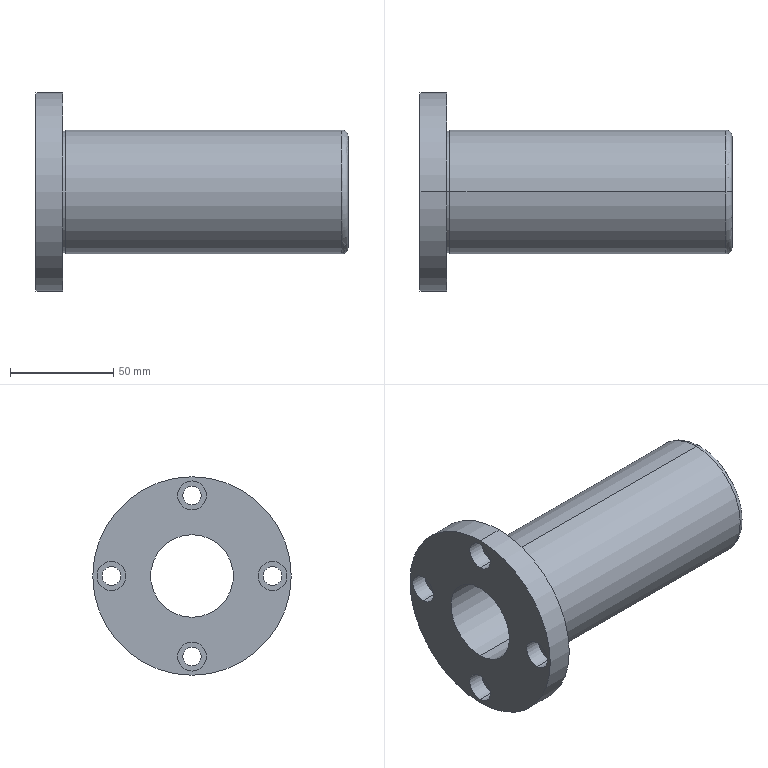Part | SolidWorks | features BaseBody 1 | 1 solid | 34 faces | box 151 x 96 x 96 mm | volume 287800 mm3 | cylinder 24 | plane 8 | torus 2 | commonest cylinder face diameters 9 x8 14 x8 40 x2 59 x2 60 x2 96 x2
STEP:
#1=CARTESIAN_POINT('',(148.,0.,30.));
#2=VERTEX_POINT('',#1);
#3=CARTESIAN_POINT('',(148.,0.,-30.));
#4=VERTEX_POINT('',#3);
#5=CARTESIAN_POINT('',(148.,0.,0.));
#6=DIRECTION('',(-1.,0.,0.));
#7=DIRECTION('',(0.,0.,1.));
#8=AXIS2_PLACEMENT_3D('',#5,#6,#7);
#9=CIRCLE('',#8,30.);
#10=EDGE_CURVE('',#2,#4,#9,.T.);
#11=ORIENTED_EDGE('',*,*,#10,.T.);
#12=CARTESIAN_POINT('',(14.5,0.,-30.));
#13=VERTEX_POINT('',#12);
#14=CARTESIAN_POINT('',(151.,0.,-30.));
#15=DIRECTION('',(-1.,0.,0.));
#16=VECTOR('',#15,1000.);
#17=LINE('',#14,#16);
#18=EDGE_CURVE('',#4,#13,#17,.T.);
#19=ORIENTED_EDGE('',*,*,#18,.T.);
#20=CARTESIAN_POINT('',(14.5,0.,30.));
#21=VERTEX_POINT('',#20);
#22=CARTESIAN_POINT('',(14.5,0.,0.));
#23=DIRECTION('',(1.,0.,0.));
#24=DIRECTION('',(0.,0.,1.));
#25=AXIS2_PLACEMENT_3D('',#22,#23,#24);
#26=CIRCLE('',#25,30.);
#27=EDGE_CURVE('',#13,#21,#26,.T.);
#28=ORIENTED_EDGE('',*,*,#27,.T.);
#29=CARTESIAN_POINT('',(151.,0.,30.));
#30=DIRECTION('',(-1.,0.,0.));
#31=VECTOR('',#30,1000.);
#32=LINE('',#29,#31);
#33=EDGE_CURVE('',#2,#21,#32,.T.);
#34=ORIENTED_EDGE('',*,*,#33,.F.);
#35=EDGE_LOOP('',(#11,#19,#28,#34));
#36=FACE_OUTER_BOUND('',#35,.T.);
#37=CARTESIAN_POINT('',(151.,0.,0.));
#38=DIRECTION('',(-1.,0.,0.));
#39=DIRECTION('',(0.,0.,1.));
#40=AXIS2_PLACEMENT_3D('',#37,#38,#39);
#41=CYLINDRICAL_SURFACE('',#40,30.);
#42=ADVANCED_FACE('',(#36),#41,.T.);
#43=ORIENTED_EDGE('',*,*,#10,.F.);
#44=CARTESIAN_POINT('',(151.,0.,27.));
#45=VERTEX_POINT('',#44);
#46=CARTESIAN_POINT('',(148.,0.,27.));
#47=DIRECTION('',(0.,1.,0.));
#48=DIRECTION('',(0.,0.,1.));
#49=AXIS2_PLACEMENT_3D('',#46,#47,#48);
#50=CIRCLE('',#49,3.);
#51=EDGE_CURVE('',#2,#45,#50,.T.);
#52=ORIENTED_EDGE('',*,*,#51,.T.);
#53=CARTESIAN_POINT('',(151.,0.,-27.));
#54=VERTEX_POINT('',#53);
#55=CARTESIAN_POINT('',(151.,0.,0.));
#56=DIRECTION('',(-1.,0.,0.));
#57=DIRECTION('',(0.,0.,-1.));
#58=AXIS2_PLACEMENT_3D('',#55,#56,#57);
#59=CIRCLE('',#58,27.);
#60=EDGE_CURVE('',#45,#54,#59,.T.);
#61=ORIENTED_EDGE('',*,*,#60,.T.);
#62=CARTESIAN_POINT('',(148.,0.,-27.));
#63=DIRECTION('',(0.,-1.,0.));
#64=DIRECTION('',(0.,0.,-1.));
#65=AXIS2_PLACEMENT_3D('',#62,#63,#64);
#66=CIRCLE('',#65,3.);
#67=EDGE_CURVE('',#4,#54,#66,.T.);
#68=ORIENTED_EDGE('',*,*,#67,.F.);
#69=EDGE_LOOP('',(#43,#52,#61,#68));
#70=FACE_OUTER_BOUND('',#69,.T.);
#71=CARTESIAN_POINT('',(148.,0.,0.));
#72=DIRECTION('',(1.,0.,0.));
#73=DIRECTION('',(0.,0.,-1.));
#74=AXIS2_PLACEMENT_3D('',#71,#72,#73);
#75=TOROIDAL_SURFACE('',#74,27.,3.);
#76=ADVANCED_FACE('',(#70),#75,.T.);
#77=CARTESIAN_POINT('',(14.5,0.,-29.5));
#78=VERTEX_POINT('',#77);
#79=CARTESIAN_POINT('',(14.5,0.,29.5));
#80=VERTEX_POINT('',#79);
#81=CARTESIAN_POINT('',(14.5,0.,0.));
#82=DIRECTION('',(1.,0.,0.));
#83=DIRECTION('',(0.,0.,1.));
#84=AXIS2_PLACEMENT_3D('',#81,#82,#83);
#85=CIRCLE('',#84,29.5);
#86=EDGE_CURVE('',#78,#80,#85,.T.);
#87=ORIENTED_EDGE('',*,*,#86,.F.);
#88=CARTESIAN_POINT('',(13.,0.,-29.5));
#89=VERTEX_POINT('',#88);
#90=CARTESIAN_POINT('',(151.,0.,-29.5));
#91=DIRECTION('',(-1.,0.,0.));
#92=VECTOR('',#91,1000.);
#93=LINE('',#90,#92);
#94=EDGE_CURVE('',#78,#89,#93,.T.);
#95=ORIENTED_EDGE('',*,*,#94,.T.);
#96=CARTESIAN_POINT('',(13.,0.,29.5));
#97=VERTEX_POINT('',#96);
#98=CARTESIAN_POINT('',(13.,0.,0.));
#99=DIRECTION('',(1.,0.,0.));
#100=DIRECTION('',(0.,0.,1.));
#101=AXIS2_PLACEMENT_3D('',#98,#99,#100);
#102=CIRCLE('',#101,29.5);
#103=EDGE_CURVE('',#89,#97,#102,.T.);
#104=ORIENTED_EDGE('',*,*,#103,.T.);
#105=CARTESIAN_POINT('',(151.,0.,29.5));
#106=DIRECTION('',(-1.,0.,0.));
#107=VECTOR('',#106,1000.);
#108=LINE('',#105,#107);
#109=EDGE_CURVE('',#80,#97,#108,.T.);
#110=ORIENTED_EDGE('',*,*,#109,.F.);
#111=EDGE_LOOP('',(#87,#95,#104,#110));
#112=FACE_OUTER_BOUND('',#111,.T.);
#113=CARTESIAN_POINT('',(151.,0.,0.));
#114=DIRECTION('',(-1.,0.,0.));
#115=DIRECTION('',(0.,0.,1.));
#116=AXIS2_PLACEMENT_3D('',#113,#114,#115);
#117=CYLINDRICAL_SURFACE('',#116,29.5);
#118=ADVANCED_FACE('',(#112),#117,.T.);
#119=CARTESIAN_POINT('',(151.,0.,-20.));
#120=VERTEX_POINT('',#119);
#121=CARTESIAN_POINT('',(151.,0.,20.));
#122=VERTEX_POINT('',#121);
#123=CARTESIAN_POINT('',(151.,0.,0.));
#124=DIRECTION('',(-1.,0.,0.));
#125=DIRECTION('',(0.,0.,1.));
#126=AXIS2_PLACEMENT_3D('',#123,#124,#125);
#127=CIRCLE('',#126,20.);
#128=EDGE_CURVE('',#120,#122,#127,.T.);
#129=ORIENTED_EDGE('',*,*,#128,.F.);
#130=CARTESIAN_POINT('',(0.,0.,-20.));
#131=VERTEX_POINT('',#130);
#132=CARTESIAN_POINT('',(151.,0.,-20.));
#133=DIRECTION('',(-1.,0.,0.));
#134=VECTOR('',#133,1000.);
#135=LINE('',#132,#134);
#136=EDGE_CURVE('',#120,#131,#135,.T.);
#137=ORIENTED_EDGE('',*,*,#136,.T.);
#138=CARTESIAN_POINT('',(0.,0.,20.));
#139=VERTEX_POINT('',#138);
#140=CARTESIAN_POINT('',(0.,0.,0.));
#141=DIRECTION('',(1.,0.,0.));
#142=DIRECTION('',(0.,0.,1.));
#143=AXIS2_PLACEMENT_3D('',#140,#141,#142);
#144=CIRCLE('',#143,20.);
#145=EDGE_CURVE('',#139,#131,#144,.T.);
#146=ORIENTED_EDGE('',*,*,#145,.F.);
#147=CARTESIAN_POINT('',(151.,0.,20.));
#148=DIRECTION('',(-1.,0.,0.));
#149=VECTOR('',#148,1000.);
#150=LINE('',#147,#149);
#151=EDGE_CURVE('',#122,#139,#150,.T.);
#152=ORIENTED_EDGE('',*,*,#151,.F.);
#153=EDGE_LOOP('',(#129,#137,#146,#152));
#154=FACE_OUTER_BOUND('',#153,.T.);
#155=CARTESIAN_POINT('',(151.,0.,0.));
#156=DIRECTION('',(-1.,0.,0.));
#157=DIRECTION('',(0.,0.,1.));
#158=AXIS2_PLACEMENT_3D('',#155,#156,#157);
#159=CYLINDRICAL_SURFACE('',#158,20.);
#160=ADVANCED_FACE('',(#154),#159,.F.);
#161=CARTESIAN_POINT('',(13.,0.,-48.));
#162=VERTEX_POINT('',#161);
#163=CARTESIAN_POINT('',(13.,0.,48.));
#164=VERTEX_POINT('',#163);
#165=CARTESIAN_POINT('',(13.,0.,0.));
#166=DIRECTION('',(1.,0.,0.));
#167=DIRECTION('',(0.,0.,1.));
#168=AXIS2_PLACEMENT_3D('',#165,#166,#167);
#169=CIRCLE('',#168,48.);
#170=EDGE_CURVE('',#162,#164,#169,.T.);
#171=ORIENTED_EDGE('',*,*,#170,.F.);
#172=CARTESIAN_POINT('',(0.,0.,-48.));
#173=VERTEX_POINT('',#172);
#174=CARTESIAN_POINT('',(151.,0.,-48.));
#175=DIRECTION('',(-1.,0.,0.));
#176=VECTOR('',#175,1000.);
#177=LINE('',#174,#176);
#178=EDGE_CURVE('',#162,#173,#177,.T.);
#179=ORIENTED_EDGE('',*,*,#178,.T.);
#180=CARTESIAN_POINT('',(0.,0.,48.));
#181=VERTEX_POINT('',#180);
#182=CARTESIAN_POINT('',(0.,0.,0.));
#183=DIRECTION('',(1.,0.,0.));
#184=DIRECTION('',(0.,0.,1.));
#185=AXIS2_PLACEMENT_3D('',#182,#183,#184);
#186=CIRCLE('',#185,48.);
#187=EDGE_CURVE('',#173,#181,#186,.T.);
#188=ORIENTED_EDGE('',*,*,#187,.T.);
#189=CARTESIAN_POINT('',(151.,0.,48.));
#190=DIRECTION('',(-1.,0.,0.));
#191=VECTOR('',#190,1000.);
#192=LINE('',#189,#191);
#193=EDGE_CURVE('',#164,#181,#192,.T.);
#194=ORIENTED_EDGE('',*,*,#193,.F.);
#195=EDGE_LOOP('',(#171,#179,#188,#194));
#196=FACE_OUTER_BOUND('',#195,.T.);
#197=CARTESIAN_POINT('',(151.,0.,0.));
#198=DIRECTION('',(-1.,0.,0.));
#199=DIRECTION('',(0.,0.,1.));
#200=AXIS2_PLACEMENT_3D('',#197,#198,#199);
#201=CYLINDRICAL_SURFACE('',#200,48.);
#202=ADVANCED_FACE('',(#196),#201,.T.);
#203=CARTESIAN_POINT('',(13.,39.,-4.5));
#204=VERTEX_POINT('',#203);
#205=CARTESIAN_POINT('',(13.,39.,4.5));
#206=VERTEX_POINT('',#205);
#207=CARTESIAN_POINT('',(13.,39.,0.));
#208=DIRECTION('',(-1.,0.,0.));
#209=DIRECTION('',(0.,0.,1.));
#210=AXIS2_PLACEMENT_3D('',#207,#208,#209);
#211=CIRCLE('',#210,4.5);
#212=EDGE_CURVE('',#204,#206,#211,.T.);
#213=ORIENTED_EDGE('',*,*,#212,.F.);
#214=CARTESIAN_POINT('',(8.1,39.,-4.5));
#215=VERTEX_POINT('',#214);
#216=CARTESIAN_POINT('',(13.,39.,-4.5));
#217=DIRECTION('',(-1.,0.,0.));
#218=VECTOR('',#217,1000.);
#219=LINE('',#216,#218);
#220=EDGE_CURVE('',#204,#215,#219,.T.);
#221=ORIENTED_EDGE('',*,*,#220,.T.);
#222=CARTESIAN_POINT('',(8.1,39.,4.5));
#223=VERTEX_POINT('',#222);
#224=CARTESIAN_POINT('',(8.1,39.,0.));
#225=DIRECTION('',(1.,0.,0.));
#226=DIRECTION('',(0.,0.,1.));
#227=AXIS2_PLACEMENT_3D('',#224,#225,#226);
#228=CIRCLE('',#227,4.5);
#229=EDGE_CURVE('',#223,#215,#228,.T.);
#230=ORIENTED_EDGE('',*,*,#229,.F.);
#231=CARTESIAN_POINT('',(13.,39.,4.5));
#232=DIRECTION('',(-1.,0.,0.));
#233=VECTOR('',#232,1000.);
#234=LINE('',#231,#233);
#235=EDGE_CURVE('',#206,#223,#234,.T.);
#236=ORIENTED_EDGE('',*,*,#235,.F.);
#237=EDGE_LOOP('',(#213,#221,#230,#236));
#238=FACE_OUTER_BOUND('',#237,.T.);
#239=CARTESIAN_POINT('',(13.,39.,0.));
#240=DIRECTION('',(-1.,0.,0.));
#241=DIRECTION('',(0.,0.,1.));
#242=AXIS2_PLACEMENT_3D('',#239,#240,#241);
#243=CYLINDRICAL_SURFACE('',#242,4.5);
#244=ADVANCED_FACE('',(#238),#243,.F.);
#245=CARTESIAN_POINT('',(13.,0.,-43.5));
#246=VERTEX_POINT('',#245);
#247=CARTESIAN_POINT('',(13.,0.,-34.5));
#248=VERTEX_POINT('',#247);
#249=CARTESIAN_POINT('',(13.,0.,-39.));
#250=DIRECTION('',(-1.,0.,0.));
#251=DIRECTION('',(0.,0.,1.));
#252=AXIS2_PLACEMENT_3D('',#249,#250,#251);
#253=CIRCLE('',#252,4.5);
#254=EDGE_CURVE('',#246,#248,#253,.T.);
#255=ORIENTED_EDGE('',*,*,#254,.F.);
#256=CARTESIAN_POINT('',(8.1,0.,-43.5));
#257=VERTEX_POINT('',#256);
#258=CARTESIAN_POINT('',(13.,0.,-43.5));
#259=DIRECTION('',(-1.,0.,0.));
#260=VECTOR('',#259,1000.);
#261=LINE('',#258,#260);
#262=EDGE_CURVE('',#246,#257,#261,.T.);
#263=ORIENTED_EDGE('',*,*,#262,.T.);
#264=CARTESIAN_POINT('',(8.1,0.,-34.5));
#265=VERTEX_POINT('',#264);
#266=CARTESIAN_POINT('',(8.1,0.,-39.));
#267=DIRECTION('',(1.,0.,0.));
#268=DIRECTION('',(0.,0.,1.));
#269=AXIS2_PLACEMENT_3D('',#266,#267,#268);
#270=CIRCLE('',#269,4.5);
#271=EDGE_CURVE('',#265,#257,#270,.T.);
#272=ORIENTED_EDGE('',*,*,#271,.F.);
#273=CARTESIAN_POINT('',(13.,0.,-34.5));
#274=DIRECTION('',(-1.,0.,0.));
#275=VECTOR('',#274,1000.);
#276=LINE('',#273,#275);
#277=EDGE_CURVE('',#248,#265,#276,.T.);
#278=ORIENTED_EDGE('',*,*,#277,.F.);
#279=EDGE_LOOP('',(#255,#263,#272,#278));
#280=FACE_OUTER_BOUND('',#279,.T.);
#281=CARTESIAN_POINT('',(13.,0.,-39.));
#282=DIRECTION('',(-1.,0.,0.));
#283=DIRECTION('',(0.,0.,1.));
#284=AXIS2_PLACEMENT_3D('',#281,#282,#283);
#285=CYLINDRICAL_SURFACE('',#284,4.5);
#286=ADVANCED_FACE('',(#280),#285,.F.);
#287=CARTESIAN_POINT('',(13.,-39.,-4.5));
#288=VERTEX_POINT('',#287);
#289=CARTESIAN_POINT('',(13.,-39.,4.5));
#290=VERTEX_POINT('',#289);
#291=CARTESIAN_POINT('',(13.,-39.,0.));
#292=DIRECTION('',(-1.,0.,0.));
#293=DIRECTION('',(0.,0.,1.));
#294=AXIS2_PLACEMENT_3D('',#291,#292,#293);
#295=CIRCLE('',#294,4.5);
#296=EDGE_CURVE('',#288,#290,#295,.T.);
#297=ORIENTED_EDGE('',*,*,#296,.F.);
#298=CARTESIAN_POINT('',(8.1,-39.,-4.5));
#299=VERTEX_POINT('',#298);
#300=CARTESIAN_POINT('',(13.,-39.,-4.5));
#301=DIRECTION('',(-1.,0.,0.));
#302=VECTOR('',#301,1000.);
#303=LINE('',#300,#302);
#304=EDGE_CURVE('',#288,#299,#303,.T.);
#305=ORIENTED_EDGE('',*,*,#304,.T.);
#306=CARTESIAN_POINT('',(8.1,-39.,4.5));
#307=VERTEX_POINT('',#306);
#308=CARTESIAN_POINT('',(8.1,-39.,0.));
#309=DIRECTION('',(1.,0.,0.));
#310=DIRECTION('',(0.,0.,1.));
#311=AXIS2_PLACEMENT_3D('',#308,#309,#310);
#312=CIRCLE('',#311,4.5);
#313=EDGE_CURVE('',#307,#299,#312,.T.);
#314=ORIENTED_EDGE('',*,*,#313,.F.);
#315=CARTESIAN_POINT('',(13.,-39.,4.5));
#316=DIRECTION('',(-1.,0.,0.));
#317=VECTOR('',#316,1000.);
#318=LINE('',#315,#317);
#319=EDGE_CURVE('',#290,#307,#318,.T.);
#320=ORIENTED_EDGE('',*,*,#319,.F.);
#321=EDGE_LOOP('',(#297,#305,#314,#320));
#322=FACE_OUTER_BOUND('',#321,.T.);
#323=CARTESIAN_POINT('',(13.,-39.,0.));
#324=DIRECTION('',(-1.,0.,0.));
#325=DIRECTION('',(0.,0.,1.));
#326=AXIS2_PLACEMENT_3D('',#323,#324,#325);
#327=CYLINDRICAL_SURFACE('',#326,4.5);
#328=ADVANCED_FACE('',(#322),#327,.F.);
#329=CARTESIAN_POINT('',(13.,0.,34.5));
#330=VERTEX_POINT('',#329);
#331=CARTESIAN_POINT('',(13.,0.,43.5));
#332=VERTEX_POINT('',#331);
#333=CARTESIAN_POINT('',(13.,0.,39.));
#334=DIRECTION('',(-1.,0.,0.));
#335=DIRECTION('',(0.,0.,1.));
#336=AXIS2_PLACEMENT_3D('',#333,#334,#335);
#337=CIRCLE('',#336,4.5);
#338=EDGE_CURVE('',#330,#332,#337,.T.);
#339=ORIENTED_EDGE('',*,*,#338,.F.);
#340=CARTESIAN_POINT('',(8.1,0.,34.5));
#341=VERTEX_POINT('',#340);
#342=CARTESIAN_POINT('',(13.,0.,34.5));
#343=DIRECTION('',(-1.,0.,0.));
#344=VECTOR('',#343,1000.);
#345=LINE('',#342,#344);
#346=EDGE_CURVE('',#330,#341,#345,.T.);
#347=ORIENTED_EDGE('',*,*,#346,.T.);
#348=CARTESIAN_POINT('',(8.1,0.,43.5));
#349=VERTEX_POINT('',#348);
#350=CARTESIAN_POINT('',(8.1,0.,39.));
#351=DIRECTION('',(1.,0.,0.));
#352=DIRECTION('',(0.,0.,1.));
#353=AXIS2_PLACEMENT_3D('',#350,#351,#352);
#354=CIRCLE('',#353,4.5);
#355=EDGE_CURVE('',#349,#341,#354,.T.);
#356=ORIENTED_EDGE('',*,*,#355,.F.);
#357=CARTESIAN_POINT('',(13.,0.,43.5));
#358=DIRECTION('',(-1.,0.,0.));
#359=VECTOR('',#358,1000.);
#360=LINE('',#357,#359);
#361=EDGE_CURVE('',#332,#349,#360,.T.);
#362=ORIENTED_EDGE('',*,*,#361,.F.);
#363=EDGE_LOOP('',(#339,#347,#356,#362));
#364=FACE_OUTER_BOUND('',#363,.T.);
#365=CARTESIAN_POINT('',(13.,0.,39.));
#366=DIRECTION('',(-1.,0.,0.));
#367=DIRECTION('',(0.,0.,1.));
#368=AXIS2_PLACEMENT_3D('',#365,#366,#367);
#369=CYLINDRICAL_SURFACE('',#368,4.5);
#370=ADVANCED_FACE('',(#364),#369,.F.);
#371=CARTESIAN_POINT('',(8.1,39.,-7.));
#372=VERTEX_POINT('',#371);
#373=CARTESIAN_POINT('',(8.1,39.,7.));
#374=VERTEX_POINT('',#373);
#375=CARTESIAN_POINT('',(8.1,39.,0.));
#376=DIRECTION('',(-1.,0.,0.));
#377=DIRECTION('',(0.,0.,1.));
#378=AXIS2_PLACEMENT_3D('',#375,#376,#377);
#379=CIRCLE('',#378,7.);
#380=EDGE_CURVE('',#372,#374,#379,.T.);
#381=ORIENTED_EDGE('',*,*,#380,.F.);
#382=CARTESIAN_POINT('',(0.,39.,-7.));
#383=VERTEX_POINT('',#382);
#384=CARTESIAN_POINT('',(13.,39.,-7.));
#385=DIRECTION('',(-1.,0.,0.));
#386=VECTOR('',#385,1000.);
#387=LINE('',#384,#386);
#388=EDGE_CURVE('',#372,#383,#387,.T.);
#389=ORIENTED_EDGE('',*,*,#388,.T.);
#390=CARTESIAN_POINT('',(0.,39.,7.));
#391=VERTEX_POINT('',#390);
#392=CARTESIAN_POINT('',(0.,39.,0.));
#393=DIRECTION('',(1.,0.,0.));
#394=DIRECTION('',(0.,0.,1.));
#395=AXIS2_PLACEMENT_3D('',#392,#393,#394);
#396=CIRCLE('',#395,7.);
#397=EDGE_CURVE('',#391,#383,#396,.T.);
#398=ORIENTED_EDGE('',*,*,#397,.F.);
#399=CARTESIAN_POINT('',(13.,39.,7.));
#400=DIRECTION('',(-1.,0.,0.));
#401=VECTOR('',#400,1000.);
#402=LINE('',#399,#401);
#403=EDGE_CURVE('',#374,#391,#402,.T.);
#404=ORIENTED_EDGE('',*,*,#403,.F.);
#405=EDGE_LOOP('',(#381,#389,#398,#404));
#406=FACE_OUTER_BOUND('',#405,.T.);
#407=CARTESIAN_POINT('',(13.,39.,0.));
#408=DIRECTION('',(-1.,0.,0.));
#409=DIRECTION('',(0.,0.,1.));
#410=AXIS2_PLACEMENT_3D('',#407,#408,#409);
#411=CYLINDRICAL_SURFACE('',#410,7.);
#412=ADVANCED_FACE('',(#406),#411,.F.);
#413=CARTESIAN_POINT('',(8.1,0.,-46.));
#414=VERTEX_POINT('',#413);
#415=CARTESIAN_POINT('',(8.1,0.,-32.));
#416=VERTEX_POINT('',#415);
#417=CARTESIAN_POINT('',(8.1,0.,-39.));
#418=DIRECTION('',(-1.,0.,0.));
#419=DIRECTION('',(0.,0.,1.));
#420=AXIS2_PLACEMENT_3D('',#417,#418,#419);
#421=CIRCLE('',#420,7.);
#422=EDGE_CURVE('',#414,#416,#421,.T.);
#423=ORIENTED_EDGE('',*,*,#422,.F.);
#424=CARTESIAN_POINT('',(0.,0.,-46.));
#425=VERTEX_POINT('',#424);
#426=CARTESIAN_POINT('',(13.,0.,-46.));
#427=DIRECTION('',(-1.,0.,0.));
#428=VECTOR('',#427,1000.);
#429=LINE('',#426,#428);
#430=EDGE_CURVE('',#414,#425,#429,.T.);
#431=ORIENTED_EDGE('',*,*,#430,.T.);
#432=CARTESIAN_POINT('',(0.,0.,-32.));
#433=VERTEX_POINT('',#432);
#434=CARTESIAN_POINT('',(0.,0.,-39.));
#435=DIRECTION('',(1.,0.,0.));
#436=DIRECTION('',(0.,0.,1.));
#437=AXIS2_PLACEMENT_3D('',#434,#435,#436);
#438=CIRCLE('',#437,7.);
#439=EDGE_CURVE('',#433,#425,#438,.T.);
#440=ORIENTED_EDGE('',*,*,#439,.F.);
#441=CARTESIAN_POINT('',(13.,0.,-32.));
#442=DIRECTION('',(-1.,0.,0.));
#443=VECTOR('',#442,1000.);
#444=LINE('',#441,#443);
#445=EDGE_CURVE('',#416,#433,#444,.T.);
#446=ORIENTED_EDGE('',*,*,#445,.F.);
#447=EDGE_LOOP('',(#423,#431,#440,#446));
#448=FACE_OUTER_BOUND('',#447,.T.);
#449=CARTESIAN_POINT('',(13.,0.,-39.));
#450=DIRECTION('',(-1.,0.,0.));
#451=DIRECTION('',(0.,0.,1.));
#452=AXIS2_PLACEMENT_3D('',#449,#450,#451);
#453=CYLINDRICAL_SURFACE('',#452,7.);
#454=ADVANCED_FACE('',(#448),#453,.F.);
#455=CARTESIAN_POINT('',(8.1,-39.,-7.));
#456=VERTEX_POINT('',#455);
#457=CARTESIAN_POINT('',(8.1,-39.,7.));
#458=VERTEX_POINT('',#457);
#459=CARTESIAN_POINT('',(8.1,-39.,0.));
#460=DIRECTION('',(-1.,0.,0.));
#461=DIRECTION('',(0.,0.,1.));
#462=AXIS2_PLACEMENT_3D('',#459,#460,#461);
#463=CIRCLE('',#462,7.);
#464=EDGE_CURVE('',#456,#458,#463,.T.);
#465=ORIENTED_EDGE('',*,*,#464,.F.);
#466=CARTESIAN_POINT('',(0.,-39.,-7.));
#467=VERTEX_POINT('',#466);
#468=CARTESIAN_POINT('',(13.,-39.,-7.));
#469=DIRECTION('',(-1.,0.,0.));
#470=VECTOR('',#469,1000.);
#471=LINE('',#468,#470);
#472=EDGE_CURVE('',#456,#467,#471,.T.);
#473=ORIENTED_EDGE('',*,*,#472,.T.);
#474=CARTESIAN_POINT('',(0.,-39.,7.));
#475=VERTEX_POINT('',#474);
#476=CARTESIAN_POINT('',(0.,-39.,0.));
#477=DIRECTION('',(1.,0.,0.));
#478=DIRECTION('',(0.,0.,1.));
#479=AXIS2_PLACEMENT_3D('',#476,#477,#478);
#480=CIRCLE('',#479,7.);
#481=EDGE_CURVE('',#475,#467,#480,.T.);
#482=ORIENTED_EDGE('',*,*,#481,.F.);
#483=CARTESIAN_POINT('',(13.,-39.,7.));
#484=DIRECTION('',(-1.,0.,0.));
#485=VECTOR('',#484,1000.);
#486=LINE('',#483,#485);
#487=EDGE_CURVE('',#458,#475,#486,.T.);
#488=ORIENTED_EDGE('',*,*,#487,.F.);
#489=EDGE_LOOP('',(#465,#473,#482,#488));
#490=FACE_OUTER_BOUND('',#489,.T.);
#491=CARTESIAN_POINT('',(13.,-39.,0.));
#492=DIRECTION('',(-1.,0.,0.));
#493=DIRECTION('',(0.,0.,1.));
#494=AXIS2_PLACEMENT_3D('',#491,#492,#493);
#495=CYLINDRICAL_SURFACE('',#494,7.);
#496=ADVANCED_FACE('',(#490),#495,.F.);
#497=CARTESIAN_POINT('',(8.1,0.,32.));
#498=VERTEX_POINT('',#497);
#499=CARTESIAN_POINT('',(8.1,0.,46.));
#500=VERTEX_POINT('',#499);
#501=CARTESIAN_POINT('',(8.1,0.,39.));
#502=DIRECTION('',(-1.,0.,0.));
#503=DIRECTION('',(0.,0.,1.));
#504=AXIS2_PLACEMENT_3D('',#501,#502,#503);
#505=CIRCLE('',#504,7.);
#506=EDGE_CURVE('',#498,#500,#505,.T.);
#507=ORIENTED_EDGE('',*,*,#506,.F.);
#508=CARTESIAN_POINT('',(0.,0.,32.));
#509=VERTEX_POINT('',#508);
#510=CARTESIAN_POINT('',(13.,0.,32.));
#511=DIRECTION('',(-1.,0.,0.));
#512=VECTOR('',#511,1000.);
#513=LINE('',#510,#512);
#514=EDGE_CURVE('',#498,#509,#513,.T.);
#515=ORIENTED_EDGE('',*,*,#514,.T.);
#516=CARTESIAN_POINT('',(0.,0.,46.));
#517=VERTEX_POINT('',#516);
#518=CARTESIAN_POINT('',(0.,0.,39.));
#519=DIRECTION('',(1.,0.,0.));
#520=DIRECTION('',(0.,0.,1.));
#521=AXIS2_PLACEMENT_3D('',#518,#519,#520);
#522=CIRCLE('',#521,7.);
#523=EDGE_CURVE('',#517,#509,#522,.T.);
#524=ORIENTED_EDGE('',*,*,#523,.F.);
#525=CARTESIAN_POINT('',(13.,0.,46.));
#526=DIRECTION('',(-1.,0.,0.));
#527=VECTOR('',#526,1000.);
#528=LINE('',#525,#527);
#529=EDGE_CURVE('',#500,#517,#528,.T.);
#530=ORIENTED_EDGE('',*,*,#529,.F.);
#531=EDGE_LOOP('',(#507,#515,#524,#530));
#532=FACE_OUTER_BOUND('',#531,.T.);
#533=CARTESIAN_POINT('',(13.,0.,39.));
#534=DIRECTION('',(-1.,0.,0.));
#535=DIRECTION('',(0.,0.,1.));
#536=AXIS2_PLACEMENT_3D('',#533,#534,#535);
#537=CYLINDRICAL_SURFACE('',#536,7.);
#538=ADVANCED_FACE('',(#532),#537,.F.);
#539=ORIENTED_EDGE('',*,*,#18,.F.);
#540=CARTESIAN_POINT('',(148.,0.,0.));
#541=DIRECTION('',(-1.,0.,0.));
#542=DIRECTION('',(0.,0.,1.));
#543=AXIS2_PLACEMENT_3D('',#540,#541,#542);
#544=CIRCLE('',#543,30.);
#545=EDGE_CURVE('',#4,#2,#544,.T.);
#546=ORIENTED_EDGE('',*,*,#545,.T.);
#547=ORIENTED_EDGE('',*,*,#33,.T.);
#548=CARTESIAN_POINT('',(14.5,0.,0.));
#549=DIRECTION('',(1.,0.,0.));
#550=DIRECTION('',(0.,0.,1.));
#551=AXIS2_PLACEMENT_3D('',#548,#549,#550);
#552=CIRCLE('',#551,30.);
#553=EDGE_CURVE('',#21,#13,#552,.T.);
#554=ORIENTED_EDGE('',*,*,#553,.T.);
#555=EDGE_LOOP('',(#539,#546,#547,#554));
#556=FACE_OUTER_BOUND('',#555,.T.);
#557=CARTESIAN_POINT('',(151.,0.,0.));
#558=DIRECTION('',(-1.,0.,0.));
#559=DIRECTION('',(0.,0.,1.));
#560=AXIS2_PLACEMENT_3D('',#557,#558,#559);
#561=CYLINDRICAL_SURFACE('',#560,30.);
#562=ADVANCED_FACE('',(#556),#561,.T.);
#563=CARTESIAN_POINT('',(14.5,0.,0.));
#564=DIRECTION('',(1.,0.,0.));
#565=DIRECTION('',(0.,0.,1.));
#566=AXIS2_PLACEMENT_3D('',#563,#564,#565);
#567=CIRCLE('',#566,29.5);
#568=EDGE_CURVE('',#80,#78,#567,.T.);
#569=ORIENTED_EDGE('',*,*,#568,.T.);
#570=ORIENTED_EDGE('',*,*,#86,.T.);
#571=EDGE_LOOP('',(#569,#570));
#572=FACE_BOUND('',#571,.T.);
#573=ORIENTED_EDGE('',*,*,#553,.F.);
#574=ORIENTED_EDGE('',*,*,#27,.F.);
#575=EDGE_LOOP('',(#573,#574));
#576=FACE_OUTER_BOUND('',#575,.T.);
#577=CARTESIAN_POINT('',(14.5,30.,0.));
#578=DIRECTION('',(-1.,0.,0.));
#579=DIRECTION('',(0.,0.,1.));
#580=AXIS2_PLACEMENT_3D('',#577,#578,#579);
#581=PLANE('',#580);
#582=ADVANCED_FACE('',(#572,#576),#581,.T.);
#583=ORIENTED_EDGE('',*,*,#51,.F.);
#584=ORIENTED_EDGE('',*,*,#545,.F.);
#585=ORIENTED_EDGE('',*,*,#67,.T.);
#586=CARTESIAN_POINT('',(151.,0.,0.));
#587=DIRECTION('',(-1.,0.,0.));
#588=DIRECTION('',(0.,0.,-1.));
#589=AXIS2_PLACEMENT_3D('',#586,#587,#588);
#590=CIRCLE('',#589,27.);
#591=EDGE_CURVE('',#54,#45,#590,.T.);
#592=ORIENTED_EDGE('',*,*,#591,.T.);
#593=EDGE_LOOP('',(#583,#584,#585,#592));
#594=FACE_OUTER_BOUND('',#593,.T.);
#595=CARTESIAN_POINT('',(148.,0.,0.));
#596=DIRECTION('',(1.,0.,0.));
#597=DIRECTION('',(0.,0.,-1.));
#598=AXIS2_PLACEMENT_3D('',#595,#596,#597);
#599=TOROIDAL_SURFACE('',#598,27.,3.);
#600=ADVANCED_FACE('',(#594),#599,.T.);
#601=ORIENTED_EDGE('',*,*,#94,.F.);
#602=ORIENTED_EDGE('',*,*,#568,.F.);
#603=ORIENTED_EDGE('',*,*,#109,.T.);
#604=CARTESIAN_POINT('',(13.,0.,0.));
#605=DIRECTION('',(1.,0.,0.));
#606=DIRECTION('',(0.,0.,1.));
#607=AXIS2_PLACEMENT_3D('',#604,#605,#606);
#608=CIRCLE('',#607,29.5);
#609=EDGE_CURVE('',#97,#89,#608,.T.);
#610=ORIENTED_EDGE('',*,*,#609,.T.);
#611=EDGE_LOOP('',(#601,#602,#603,#610));
#612=FACE_OUTER_BOUND('',#611,.T.);
#613=CARTESIAN_POINT('',(151.,0.,0.));
#614=DIRECTION('',(-1.,0.,0.));
#615=DIRECTION('',(0.,0.,1.));
#616=AXIS2_PLACEMENT_3D('',#613,#614,#615);
#617=CYLINDRICAL_SURFACE('',#616,29.5);
#618=ADVANCED_FACE('',(#612),#617,.T.);
#619=ORIENTED_EDGE('',*,*,#591,.F.);
#620=ORIENTED_EDGE('',*,*,#60,.F.);
#621=EDGE_LOOP('',(#619,#620));
#622=FACE_OUTER_BOUND('',#621,.T.);
#623=CARTESIAN_POINT('',(151.,0.,0.));
#624=DIRECTION('',(-1.,0.,0.));
#625=DIRECTION('',(0.,0.,1.));
#626=AXIS2_PLACEMENT_3D('',#623,#624,#625);
#627=CIRCLE('',#626,20.);
#628=EDGE_CURVE('',#122,#120,#627,.T.);
#629=ORIENTED_EDGE('',*,*,#628,.T.);
#630=ORIENTED_EDGE('',*,*,#128,.T.);
#631=EDGE_LOOP('',(#629,#630));
#632=FACE_BOUND('',#631,.T.);
#633=CARTESIAN_POINT('',(151.,20.,0.));
#634=DIRECTION('',(1.,0.,0.));
#635=DIRECTION('',(0.,0.,-1.));
#636=AXIS2_PLACEMENT_3D('',#633,#634,#635);
#637=PLANE('',#636);
#638=ADVANCED_FACE('',(#622,#632),#637,.T.);
#639=CARTESIAN_POINT('',(13.,0.,0.));
#640=DIRECTION('',(1.,0.,0.));
#641=DIRECTION('',(0.,0.,1.));
#642=AXIS2_PLACEMENT_3D('',#639,#640,#641);
#643=CIRCLE('',#642,48.);
#644=EDGE_CURVE('',#164,#162,#643,.T.);
#645=ORIENTED_EDGE('',*,*,#644,.T.);
#646=ORIENTED_EDGE('',*,*,#170,.T.);
#647=EDGE_LOOP('',(#645,#646));
#648=FACE_OUTER_BOUND('',#647,.T.);
#649=CARTESIAN_POINT('',(13.,39.,0.));
#650=DIRECTION('',(-1.,0.,0.));
#651=DIRECTION('',(0.,0.,1.));
#652=AXIS2_PLACEMENT_3D('',#649,#650,#651);
#653=CIRCLE('',#652,4.5);
#654=EDGE_CURVE('',#206,#204,#653,.T.);
#655=ORIENTED_EDGE('',*,*,#654,.T.);
#656=ORIENTED_EDGE('',*,*,#212,.T.);
#657=EDGE_LOOP('',(#655,#656));
#658=FACE_BOUND('',#657,.T.);
#659=CARTESIAN_POINT('',(13.,0.,-39.));
#660=DIRECTION('',(-1.,0.,0.));
#661=DIRECTION('',(0.,0.,1.));
#662=AXIS2_PLACEMENT_3D('',#659,#660,#661);
#663=CIRCLE('',#662,4.5);
#664=EDGE_CURVE('',#248,#246,#663,.T.);
#665=ORIENTED_EDGE('',*,*,#664,.T.);
#666=ORIENTED_EDGE('',*,*,#254,.T.);
#667=EDGE_LOOP('',(#665,#666));
#668=FACE_BOUND('',#667,.T.);
#669=ORIENTED_EDGE('',*,*,#609,.F.);
#670=ORIENTED_EDGE('',*,*,#103,.F.);
#671=EDGE_LOOP('',(#669,#670));
#672=FACE_BOUND('',#671,.T.);
#673=CARTESIAN_POINT('',(13.,-39.,0.));
#674=DIRECTION('',(-1.,0.,0.));
#675=DIRECTION('',(0.,0.,1.));
#676=AXIS2_PLACEMENT_3D('',#673,#674,#675);
#677=CIRCLE('',#676,4.5);
#678=EDGE_CURVE('',#290,#288,#677,.T.);
#679=ORIENTED_EDGE('',*,*,#678,.T.);
#680=ORIENTED_EDGE('',*,*,#296,.T.);
#681=EDGE_LOOP('',(#679,#680));
#682=FACE_BOUND('',#681,.T.);
#683=CARTESIAN_POINT('',(13.,0.,39.));
#684=DIRECTION('',(-1.,0.,0.));
#685=DIRECTION('',(0.,0.,1.));
#686=AXIS2_PLACEMENT_3D('',#683,#684,#685);
#687=CIRCLE('',#686,4.5);
#688=EDGE_CURVE('',#332,#330,#687,.T.);
#689=ORIENTED_EDGE('',*,*,#688,.T.);
#690=ORIENTED_EDGE('',*,*,#338,.T.);
#691=EDGE_LOOP('',(#689,#690));
#692=FACE_BOUND('',#691,.T.);
#693=CARTESIAN_POINT('',(13.,29.5,0.));
#694=DIRECTION('',(1.,0.,0.));
#695=DIRECTION('',(0.,0.,-1.));
#696=AXIS2_PLACEMENT_3D('',#693,#694,#695);
#697=PLANE('',#696);
#698=ADVANCED_FACE('',(#648,#658,#668,#672,#682,#692),#697,.T.);
#699=ORIENTED_EDGE('',*,*,#136,.F.);
#700=ORIENTED_EDGE('',*,*,#628,.F.);
#701=ORIENTED_EDGE('',*,*,#151,.T.);
#702=CARTESIAN_POINT('',(0.,0.,0.));
#703=DIRECTION('',(1.,0.,0.));
#704=DIRECTION('',(0.,0.,1.));
#705=AXIS2_PLACEMENT_3D('',#702,#703,#704);
#706=CIRCLE('',#705,20.);
#707=EDGE_CURVE('',#131,#139,#706,.T.);
#708=ORIENTED_EDGE('',*,*,#707,.F.);
#709=EDGE_LOOP('',(#699,#700,#701,#708));
#710=FACE_OUTER_BOUND('',#709,.T.);
#711=CARTESIAN_POINT('',(151.,0.,0.));
#712=DIRECTION('',(-1.,0.,0.));
#713=DIRECTION('',(0.,0.,1.));
#714=AXIS2_PLACEMENT_3D('',#711,#712,#713);
#715=CYLINDRICAL_SURFACE('',#714,20.);
#716=ADVANCED_FACE('',(#710),#715,.F.);
#717=ORIENTED_EDGE('',*,*,#178,.F.);
#718=ORIENTED_EDGE('',*,*,#644,.F.);
#719=ORIENTED_EDGE('',*,*,#193,.T.);
#720=CARTESIAN_POINT('',(0.,0.,0.));
#721=DIRECTION('',(1.,0.,0.));
#722=DIRECTION('',(0.,0.,1.));
#723=AXIS2_PLACEMENT_3D('',#720,#721,#722);
#724=CIRCLE('',#723,48.);
#725=EDGE_CURVE('',#181,#173,#724,.T.);
#726=ORIENTED_EDGE('',*,*,#725,.T.);
#727=EDGE_LOOP('',(#717,#718,#719,#726));
#728=FACE_OUTER_BOUND('',#727,.T.);
#729=CARTESIAN_POINT('',(151.,0.,0.));
#730=DIRECTION('',(-1.,0.,0.));
#731=DIRECTION('',(0.,0.,1.));
#732=AXIS2_PLACEMENT_3D('',#729,#730,#731);
#733=CYLINDRICAL_SURFACE('',#732,48.);
#734=ADVANCED_FACE('',(#728),#733,.T.);
#735=ORIENTED_EDGE('',*,*,#220,.F.);
#736=ORIENTED_EDGE('',*,*,#654,.F.);
#737=ORIENTED_EDGE('',*,*,#235,.T.);
#738=CARTESIAN_POINT('',(8.1,39.,0.));
#739=DIRECTION('',(1.,0.,0.));
#740=DIRECTION('',(0.,0.,1.));
#741=AXIS2_PLACEMENT_3D('',#738,#739,#740);
#742=CIRCLE('',#741,4.5);
#743=EDGE_CURVE('',#215,#223,#742,.T.);
#744=ORIENTED_EDGE('',*,*,#743,.F.);
#745=EDGE_LOOP('',(#735,#736,#737,#744));
#746=FACE_OUTER_BOUND('',#745,.T.);
#747=CARTESIAN_POINT('',(13.,39.,0.));
#748=DIRECTION('',(-1.,0.,0.));
#749=DIRECTION('',(0.,0.,1.));
#750=AXIS2_PLACEMENT_3D('',#747,#748,#749);
#751=CYLINDRICAL_SURFACE('',#750,4.5);
#752=ADVANCED_FACE('',(#746),#751,.F.);
#753=ORIENTED_EDGE('',*,*,#262,.F.);
#754=ORIENTED_EDGE('',*,*,#664,.F.);
#755=ORIENTED_EDGE('',*,*,#277,.T.);
#756=CARTESIAN_POINT('',(8.1,0.,-39.));
#757=DIRECTION('',(1.,0.,0.));
#758=DIRECTION('',(0.,0.,1.));
#759=AXIS2_PLACEMENT_3D('',#756,#757,#758);
#760=CIRCLE('',#759,4.5);
#761=EDGE_CURVE('',#257,#265,#760,.T.);
#762=ORIENTED_EDGE('',*,*,#761,.F.);
#763=EDGE_LOOP('',(#753,#754,#755,#762));
#764=FACE_OUTER_BOUND('',#763,.T.);
#765=CARTESIAN_POINT('',(13.,0.,-39.));
#766=DIRECTION('',(-1.,0.,0.));
#767=DIRECTION('',(0.,0.,1.));
#768=AXIS2_PLACEMENT_3D('',#765,#766,#767);
#769=CYLINDRICAL_SURFACE('',#768,4.5);
#770=ADVANCED_FACE('',(#764),#769,.F.);
#771=ORIENTED_EDGE('',*,*,#304,.F.);
#772=ORIENTED_EDGE('',*,*,#678,.F.);
#773=ORIENTED_EDGE('',*,*,#319,.T.);
#774=CARTESIAN_POINT('',(8.1,-39.,0.));
#775=DIRECTION('',(1.,0.,0.));
#776=DIRECTION('',(0.,0.,1.));
#777=AXIS2_PLACEMENT_3D('',#774,#775,#776);
#778=CIRCLE('',#777,4.5);
#779=EDGE_CURVE('',#299,#307,#778,.T.);
#780=ORIENTED_EDGE('',*,*,#779,.F.);
#781=EDGE_LOOP('',(#771,#772,#773,#780));
#782=FACE_OUTER_BOUND('',#781,.T.);
#783=CARTESIAN_POINT('',(13.,-39.,0.));
#784=DIRECTION('',(-1.,0.,0.));
#785=DIRECTION('',(0.,0.,1.));
#786=AXIS2_PLACEMENT_3D('',#783,#784,#785);
#787=CYLINDRICAL_SURFACE('',#786,4.5);
#788=ADVANCED_FACE('',(#782),#787,.F.);
#789=ORIENTED_EDGE('',*,*,#346,.F.);
#790=ORIENTED_EDGE('',*,*,#688,.F.);
#791=ORIENTED_EDGE('',*,*,#361,.T.);
#792=CARTESIAN_POINT('',(8.1,0.,39.));
#793=DIRECTION('',(1.,0.,0.));
#794=DIRECTION('',(0.,0.,1.));
#795=AXIS2_PLACEMENT_3D('',#792,#793,#794);
#796=CIRCLE('',#795,4.5);
#797=EDGE_CURVE('',#341,#349,#796,.T.);
#798=ORIENTED_EDGE('',*,*,#797,.F.);
#799=EDGE_LOOP('',(#789,#790,#791,#798));
#800=FACE_OUTER_BOUND('',#799,.T.);
#801=CARTESIAN_POINT('',(13.,0.,39.));
#802=DIRECTION('',(-1.,0.,0.));
#803=DIRECTION('',(0.,0.,1.));
#804=AXIS2_PLACEMENT_3D('',#801,#802,#803);
#805=CYLINDRICAL_SURFACE('',#804,4.5);
#806=ADVANCED_FACE('',(#800),#805,.F.);
#807=ORIENTED_EDGE('',*,*,#145,.T.);
#808=ORIENTED_EDGE('',*,*,#707,.T.);
#809=EDGE_LOOP('',(#807,#808));
#810=FACE_BOUND('',#809,.T.);
#811=ORIENTED_EDGE('',*,*,#397,.T.);
#812=CARTESIAN_POINT('',(0.,39.,0.));
#813=DIRECTION('',(1.,0.,0.));
#814=DIRECTION('',(0.,0.,1.));
#815=AXIS2_PLACEMENT_3D('',#812,#813,#814);
#816=CIRCLE('',#815,7.);
#817=EDGE_CURVE('',#383,#391,#816,.T.);
#818=ORIENTED_EDGE('',*,*,#817,.T.);
#819=EDGE_LOOP('',(#811,#818));
#820=FACE_BOUND('',#819,.T.);
#821=ORIENTED_EDGE('',*,*,#439,.T.);
#822=CARTESIAN_POINT('',(0.,0.,-39.));
#823=DIRECTION('',(1.,0.,0.));
#824=DIRECTION('',(0.,0.,1.));
#825=AXIS2_PLACEMENT_3D('',#822,#823,#824);
#826=CIRCLE('',#825,7.);
#827=EDGE_CURVE('',#425,#433,#826,.T.);
#828=ORIENTED_EDGE('',*,*,#827,.T.);
#829=EDGE_LOOP('',(#821,#828));
#830=FACE_BOUND('',#829,.T.);
#831=ORIENTED_EDGE('',*,*,#725,.F.);
#832=ORIENTED_EDGE('',*,*,#187,.F.);
#833=EDGE_LOOP('',(#831,#832));
#834=FACE_OUTER_BOUND('',#833,.T.);
#835=ORIENTED_EDGE('',*,*,#481,.T.);
#836=CARTESIAN_POINT('',(0.,-39.,0.));
#837=DIRECTION('',(1.,0.,0.));
#838=DIRECTION('',(0.,0.,1.));
#839=AXIS2_PLACEMENT_3D('',#836,#837,#838);
#840=CIRCLE('',#839,7.);
#841=EDGE_CURVE('',#467,#475,#840,.T.);
#842=ORIENTED_EDGE('',*,*,#841,.T.);
#843=EDGE_LOOP('',(#835,#842));
#844=FACE_BOUND('',#843,.T.);
#845=ORIENTED_EDGE('',*,*,#523,.T.);
#846=CARTESIAN_POINT('',(0.,0.,39.));
#847=DIRECTION('',(1.,0.,0.));
#848=DIRECTION('',(0.,0.,1.));
#849=AXIS2_PLACEMENT_3D('',#846,#847,#848);
#850=CIRCLE('',#849,7.);
#851=EDGE_CURVE('',#509,#517,#850,.T.);
#852=ORIENTED_EDGE('',*,*,#851,.T.);
#853=EDGE_LOOP('',(#845,#852));
#854=FACE_BOUND('',#853,.T.);
#855=CARTESIAN_POINT('',(0.,48.,0.));
#856=DIRECTION('',(-1.,0.,0.));
#857=DIRECTION('',(0.,0.,1.));
#858=AXIS2_PLACEMENT_3D('',#855,#856,#857);
#859=PLANE('',#858);
#860=ADVANCED_FACE('',(#810,#820,#830,#834,#844,#854),#859,.T.);
#861=ORIENTED_EDGE('',*,*,#229,.T.);
#862=ORIENTED_EDGE('',*,*,#743,.T.);
#863=EDGE_LOOP('',(#861,#862));
#864=FACE_BOUND('',#863,.T.);
#865=CARTESIAN_POINT('',(8.1,39.,0.));
#866=DIRECTION('',(-1.,0.,0.));
#867=DIRECTION('',(0.,0.,1.));
#868=AXIS2_PLACEMENT_3D('',#865,#866,#867);
#869=CIRCLE('',#868,7.);
#870=EDGE_CURVE('',#374,#372,#869,.T.);
#871=ORIENTED_EDGE('',*,*,#870,.T.);
#872=ORIENTED_EDGE('',*,*,#380,.T.);
#873=EDGE_LOOP('',(#871,#872));
#874=FACE_OUTER_BOUND('',#873,.T.);
#875=CARTESIAN_POINT('',(8.1,46.,0.));
#876=DIRECTION('',(-1.,0.,0.));
#877=DIRECTION('',(0.,0.,1.));
#878=AXIS2_PLACEMENT_3D('',#875,#876,#877);
#879=PLANE('',#878);
#880=ADVANCED_FACE('',(#864,#874),#879,.T.);
#881=ORIENTED_EDGE('',*,*,#271,.T.);
#882=ORIENTED_EDGE('',*,*,#761,.T.);
#883=EDGE_LOOP('',(#881,#882));
#884=FACE_BOUND('',#883,.T.);
#885=CARTESIAN_POINT('',(8.1,0.,-39.));
#886=DIRECTION('',(-1.,0.,0.));
#887=DIRECTION('',(0.,0.,1.));
#888=AXIS2_PLACEMENT_3D('',#885,#886,#887);
#889=CIRCLE('',#888,7.);
#890=EDGE_CURVE('',#416,#414,#889,.T.);
#891=ORIENTED_EDGE('',*,*,#890,.T.);
#892=ORIENTED_EDGE('',*,*,#422,.T.);
#893=EDGE_LOOP('',(#891,#892));
#894=FACE_OUTER_BOUND('',#893,.T.);
#895=CARTESIAN_POINT('',(8.1,0.,-46.));
#896=DIRECTION('',(-1.,0.,0.));
#897=DIRECTION('',(0.,0.,1.));
#898=AXIS2_PLACEMENT_3D('',#895,#896,#897);
#899=PLANE('',#898);
#900=ADVANCED_FACE('',(#884,#894),#899,.T.);
#901=ORIENTED_EDGE('',*,*,#313,.T.);
#902=ORIENTED_EDGE('',*,*,#779,.T.);
#903=EDGE_LOOP('',(#901,#902));
#904=FACE_BOUND('',#903,.T.);
#905=CARTESIAN_POINT('',(8.1,-39.,0.));
#906=DIRECTION('',(-1.,0.,0.));
#907=DIRECTION('',(0.,0.,1.));
#908=AXIS2_PLACEMENT_3D('',#905,#906,#907);
#909=CIRCLE('',#908,7.);
#910=EDGE_CURVE('',#458,#456,#909,.T.);
#911=ORIENTED_EDGE('',*,*,#910,.T.);
#912=ORIENTED_EDGE('',*,*,#464,.T.);
#913=EDGE_LOOP('',(#911,#912));
#914=FACE_OUTER_BOUND('',#913,.T.);
#915=CARTESIAN_POINT('',(8.1,-32.,0.));
#916=DIRECTION('',(-1.,0.,0.));
#917=DIRECTION('',(0.,0.,1.));
#918=AXIS2_PLACEMENT_3D('',#915,#916,#917);
#919=PLANE('',#918);
#920=ADVANCED_FACE('',(#904,#914),#919,.T.);
#921=ORIENTED_EDGE('',*,*,#355,.T.);
#922=ORIENTED_EDGE('',*,*,#797,.T.);
#923=EDGE_LOOP('',(#921,#922));
#924=FACE_BOUND('',#923,.T.);
#925=CARTESIAN_POINT('',(8.1,0.,39.));
#926=DIRECTION('',(-1.,0.,0.));
#927=DIRECTION('',(0.,0.,1.));
#928=AXIS2_PLACEMENT_3D('',#925,#926,#927);
#929=CIRCLE('',#928,7.);
#930=EDGE_CURVE('',#500,#498,#929,.T.);
#931=ORIENTED_EDGE('',*,*,#930,.T.);
#932=ORIENTED_EDGE('',*,*,#506,.T.);
#933=EDGE_LOOP('',(#931,#932));
#934=FACE_OUTER_BOUND('',#933,.T.);
#935=CARTESIAN_POINT('',(8.1,0.,32.));
#936=DIRECTION('',(-1.,0.,0.));
#937=DIRECTION('',(0.,0.,1.));
#938=AXIS2_PLACEMENT_3D('',#935,#936,#937);
#939=PLANE('',#938);
#940=ADVANCED_FACE('',(#924,#934),#939,.T.);
#941=ORIENTED_EDGE('',*,*,#388,.F.);
#942=ORIENTED_EDGE('',*,*,#870,.F.);
#943=ORIENTED_EDGE('',*,*,#403,.T.);
#944=ORIENTED_EDGE('',*,*,#817,.F.);
#945=EDGE_LOOP('',(#941,#942,#943,#944));
#946=FACE_OUTER_BOUND('',#945,.T.);
#947=CARTESIAN_POINT('',(13.,39.,0.));
#948=DIRECTION('',(-1.,0.,0.));
#949=DIRECTION('',(0.,0.,1.));
#950=AXIS2_PLACEMENT_3D('',#947,#948,#949);
#951=CYLINDRICAL_SURFACE('',#950,7.);
#952=ADVANCED_FACE('',(#946),#951,.F.);
#953=ORIENTED_EDGE('',*,*,#430,.F.);
#954=ORIENTED_EDGE('',*,*,#890,.F.);
#955=ORIENTED_EDGE('',*,*,#445,.T.);
#956=ORIENTED_EDGE('',*,*,#827,.F.);
#957=EDGE_LOOP('',(#953,#954,#955,#956));
#958=FACE_OUTER_BOUND('',#957,.T.);
#959=CARTESIAN_POINT('',(13.,0.,-39.));
#960=DIRECTION('',(-1.,0.,0.));
#961=DIRECTION('',(0.,0.,1.));
#962=AXIS2_PLACEMENT_3D('',#959,#960,#961);
#963=CYLINDRICAL_SURFACE('',#962,7.);
#964=ADVANCED_FACE('',(#958),#963,.F.);
#965=ORIENTED_EDGE('',*,*,#472,.F.);
#966=ORIENTED_EDGE('',*,*,#910,.F.);
#967=ORIENTED_EDGE('',*,*,#487,.T.);
#968=ORIENTED_EDGE('',*,*,#841,.F.);
#969=EDGE_LOOP('',(#965,#966,#967,#968));
#970=FACE_OUTER_BOUND('',#969,.T.);
#971=CARTESIAN_POINT('',(13.,-39.,0.));
#972=DIRECTION('',(-1.,0.,0.));
#973=DIRECTION('',(0.,0.,1.));
#974=AXIS2_PLACEMENT_3D('',#971,#972,#973);
#975=CYLINDRICAL_SURFACE('',#974,7.);
#976=ADVANCED_FACE('',(#970),#975,.F.);
#977=ORIENTED_EDGE('',*,*,#514,.F.);
#978=ORIENTED_EDGE('',*,*,#930,.F.);
#979=ORIENTED_EDGE('',*,*,#529,.T.);
#980=ORIENTED_EDGE('',*,*,#851,.F.);
#981=EDGE_LOOP('',(#977,#978,#979,#980));
#982=FACE_OUTER_BOUND('',#981,.T.);
#983=CARTESIAN_POINT('',(13.,0.,39.));
#984=DIRECTION('',(-1.,0.,0.));
#985=DIRECTION('',(0.,0.,1.));
#986=AXIS2_PLACEMENT_3D('',#983,#984,#985);
#987=CYLINDRICAL_SURFACE('',#986,7.);
#988=ADVANCED_FACE('',(#982),#987,.F.);
#989=CLOSED_SHELL('',(#42,#76,#118,#160,#202,#244,#286,#328,#370,#412,#454,#496,#538,#562,#582,#600,#618,#638,#698,#716,#734,#752,#770,#788,#806,#860,#880,#900,#920,#940,#952,#964,#976,#988));
#990=MANIFOLD_SOLID_BREP('',#989);
#991=CARTESIAN_POINT('',(0.,0.,0.));
#992=DIRECTION('',(0.,0.,1.));
#993=DIRECTION('',(1.,0.,0.));
#994=AXIS2_PLACEMENT_3D('',#991,#992,#993);
#995=(LENGTH_UNIT()NAMED_UNIT(*)SI_UNIT(.MILLI.,.METRE.));
#996=UNCERTAINTY_MEASURE_WITH_UNIT(LENGTH_MEASURE(0.00001),#995,'','');
#997=(NAMED_UNIT(*)PLANE_ANGLE_UNIT()SI_UNIT($,.RADIAN.));
#998=(NAMED_UNIT(*)SI_UNIT($,.STERADIAN.)SOLID_ANGLE_UNIT());
#999=(GEOMETRIC_REPRESENTATION_CONTEXT(3)GLOBAL_UNCERTAINTY_ASSIGNED_CONTEXT((#996))GLOBAL_UNIT_ASSIGNED_CONTEXT((#995,#997,#998))REPRESENTATION_CONTEXT('',''));
#1000=ADVANCED_BREP_SHAPE_REPRESENTATION('',(#990,#994),#999);